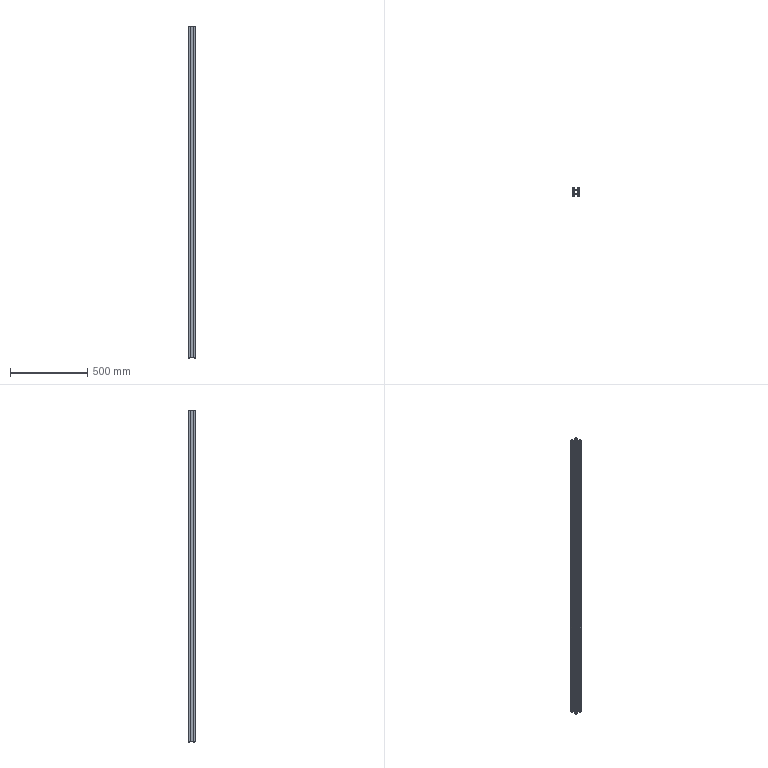Part | STEP file | 46A-00006CC11-2150mm-2 | 1 solid | 142 faces | box 50 x 50 x 2150 mm | volume 1263109 mm3 | cylinder 84 | plane 58 | commonest cylinder face diameters 1 x24 4 x24 1.5 x16 3.7 x8 6.7 x8 2 x4